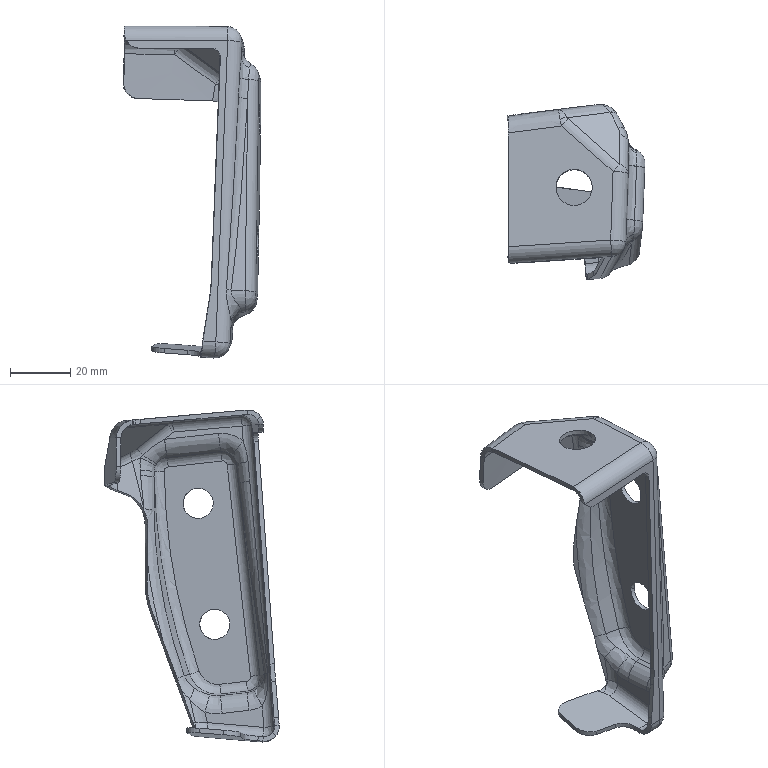Part | 1 solid | 178 faces | box 45.6 x 57.683 x 109.831 mm | volume 11972 mm3 | spline 110 | cylinder 41 | plane 20 | sphere 6 | other 1 | commonest cylinder face diameters 10 x17 7 x12 20 x3 12 x2 17 x2 100 x2